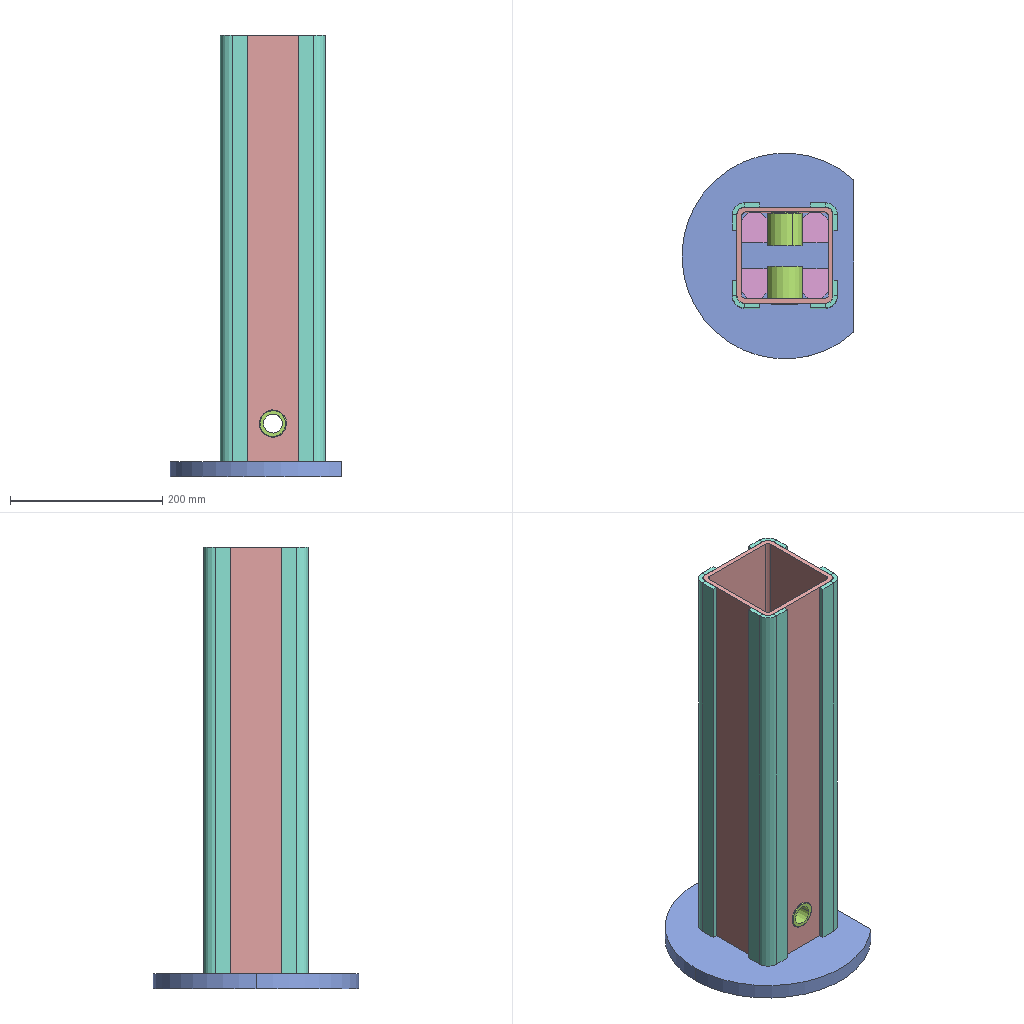Assembly | SolidWorks | 5 different items | 12 placed | box 226 x 269 x 580 mm
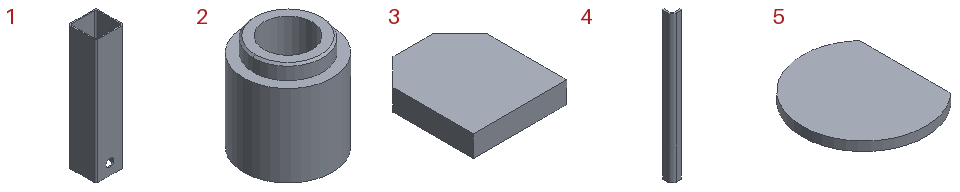Parts list (item | quantity | size | volume | features):
1 | x1 | 126 x 126 x 560 mm | 1581838 mm3 | features Fillet 2, Extrusion 1, ICE 1
2 | x2 | 46 x 46 x 50 mm | 53666 mm3 | features ICE 2, Chamfer 1, Extrusion 1
3 | x4 | 35 x 40 x 8 mm | 10400 mm3 | features Extrusion 1
4 | x4 | 36 x 36 x 560 mm | 203012 mm3 | features FlatPattern 1, SMBaseFlange 1, SheetMetal 1
5 | x1 | 225.69 x 270 x 20 mm | 1022431 mm3 | features Extrusion 1
Mates (type | each side: item.copy, entity, surface, feature):
Coincident | 1.1 face plane Boss-Extrude1 | 5.1 face plane Boss-Extrude1
DistanceDim | 5.1 select_type:24 | 1.1 face plane Boss-Extrude1 | 2 times
Concentric | 1.1 edge | 2.1 edge
Concentric | 2.1 face cylinder Boss-Extrude1 | 2.2 edge
DistanceDim | 2.1 face plane Boss-Extrude1 | 2.2 face plane Boss-Extrude1
DistanceDim | 3.1 face plane Boss-Extrude1 | 1.1 face plane Boss-Extrude1
Coincident | 1.1 face plane Boss-Extrude1 | 3.1 face plane Boss-Extrude1 | 2 times
Coincident | 3.1 face plane Boss-Extrude1 | 3.2 face plane Boss-Extrude1 | 2 times
Coincident | 1.1 face plane Boss-Extrude1 | 3.2 face plane Boss-Extrude1
Coincident | 3.3 face plane Boss-Extrude1 | 3.4 face plane Boss-Extrude1 | 2 times
Coincident | 1.1 face plane Boss-Extrude1 | 3.3 face plane Boss-Extrude1 | 2 times
Coincident | 3.2 face plane Boss-Extrude1 | 3.3 face plane Boss-Extrude1
Coincident | 1.1 face plane Boss-Extrude1 | 3.4 face plane Boss-Extrude1
Coincident | 1.1 face plane Boss-Extrude1 | 4.1 face plane Base-Flange1 | 3 times
Coincident | 4.2 face plane Base-Flange1 | 4.3 face plane Base-Flange1
Coincident | 1.1 face plane Boss-Extrude1 | 4.2 face plane Base-Flange1 | 3 times
Coincident | 4.1 face plane Base-Flange1 | 4.2 face plane Base-Flange1
Coincident | 1.1 face plane Boss-Extrude1 | 4.3 face plane Base-Flange1 | 2 times
Coincident | 1.1 face plane Boss-Extrude1 | 4.4 face plane Base-Flange1 | 2 times
Coincident | 4.1 face plane Base-Flange1 | 4.4 face plane Base-Flange1
DistanceDim | 2.2 face plane Boss-Extrude1 | 1.1 face plane Boss-Extrude1